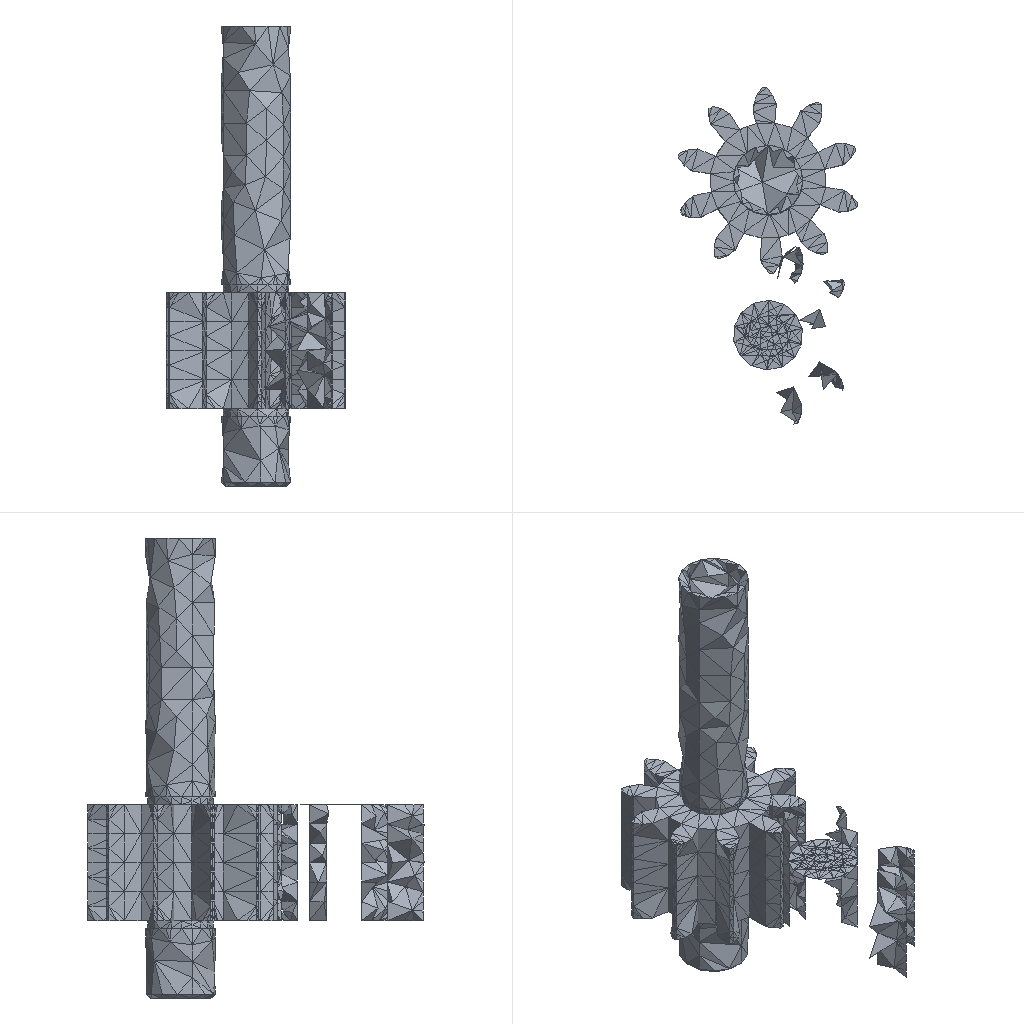Simulation study | ansys workbench
Ansys APDL input file, long lists of numbers shortened:
/batch
/config,noeldb,1     ! force off writing results to database
*get,_wallstrt,active,,time,wall
! ANSYS input file written by Workbench version 2022 R1
/assign,rstp,file,rst              ! Force Eigen analysis to write to file.rst because WB expects it
/solu
antype,,restart,,,perturbation
*DIM,_wb_ProjectScratch_dir_Modal,string,248
_wb_ProjectScratch_dir_Modal(1)= 'C:\_____\_____________\_______\_____\____\________________________\_______________\_______\_
*DIM,_wb_SolverFiles_dir_Modal,string,248
_wb_SolverFiles_dir_Modal(1)= 'C:\_____\_____________\_______\_____\____\________________________\___________\___\_____\____\_
*DIM,_wb_userfiles_dir_Modal,string,248
_wb_userfiles_dir_Modal(1)= 'C:\_____\_____________\_______\_____\____\________________________\___________\__________\_
/title,wbnew--__ (C5)
! ****** Begin Custom Load Command Snippet ******
/COM, ACT Extensions:
/COM,     LSDYNA, 2021.1
/COM,
! ****** End   Custom Load Command Snippet ******
perturb,modal,,CURRENT,DZEROKEEP          ! pre-stress modal analysis, only keep zero bcs in case future MSUP
solve, elform                                       ! Generate matrices needed for perturbation analysis
_thickRatio=0.75    ! Ratio of thick parts in the model
modopt,lanb,6
outres,erase
outres,all,none
outres,nsol,all
outres,etmp,all
mxpand                    ! default expand in case of complex solution
dmpopt,esav,no
dmpopt,emat,no
dmpopt,full,no
! *********** WB SOLVE COMMAND ***********
! check interactive state
*get,ANSINTER_,active,,int
*if,ANSINTER_,ne,0,then
/eof
*endif
solve
/com *************** Write FE CONNECTORS *********
CEWRITE,file,ce,,INTE
*get,_nmodalsolproc,active,0,numcpu
fini
/nopr
*get,_numnode,node,0,count
*get,_numelem,elem,0,count
*get, _MAXELEMNUM, elem, 0, NUM, MAX
*get, _MAXNODENUM, node, 0, NUM, MAX,,,INTERNAL
*get, _MAXELEMTYPE, etyp, 0, NUM, MAX
*get, _MAXREALCONST, real, 0, NUM, MAX
/gopr
*get,_wallasol,active,,time,wall
/post1
/nopr
*dim,_direction,CHAR,6,1
_direction(1) = 'X'
_direction(2) = 'Y'
_direction(3) = 'Z'
_direction(4) = 'ROTX'
_direction(5) = 'ROTY'
_direction(6) = 'ROTZ'
*get,_lastLS,active,0,set,LSTP
*get,_beginset,active,0,set,nset,first,_lastLS
*get,_endset,active,0,set,nset,last,_lastLS
_nummodes = 0
*if,_endset,gt,0,then
_nummodes = _endset - _beginset + 1
*endif
*do,i_mode,1,_nummodes
   *do,j_component,1,6
			*get,PFACT_%i_mode%_%j_component%,MODE,%i_mode%,PFACT,,DIREC,_direction(%j_component%)
   *enddo
*enddo
*dim,_tmdirection,CHAR,6,1
_tmdirection(1) = 'X'
_tmdirection(2) = 'Y'
_tmdirection(3) = 'Z'
_tmdirection(4) = 'X'
_tmdirection(5) = 'Y'
_tmdirection(6) = 'Z'
*do,j_component,1,6
    *if,j_component,gt,3,then
        *get,TOTALMASS_%j_component%,ELEM,0,IOR,_tmdirection(%j_component%)
    *else
        *get,TOTALMASS_%j_component%,ELEM,0,MTOT,_tmdirection(%j_component%)
    *endif
*enddo
/gopr
xmlo,ENCODING,ISO-8859-1
xmlo,parm
/xml,parm,xml
fini
/gopr
*get,_walldone,active,,time,wall
_preptime=(_wallbsol-_wallstrt)*3600
_solvtime=(_wallasol-_wallbsol)*3600
_posttime=(_walldone-_wallasol)*3600
_totaltim=(_walldone-_wallstrt)*3600
*get,_dlbratio,active,0,solu,dlbr
*get,_combtime,active,0,solu,comb
*get,_ssmode,active,0,solu,ssmm
*get,_ndofs,active,0,solu,ndof
/fclean				!clean distributed files
/com,--- Total number of nodes = %_numnode%
/com,--- Total number of elements = %_numelem%
/com,--- Element load balance ratio = %_dlbratio%
/com,--- Time to combine distributed files = %_combtime%
/com,--- Sparse memory mode = %_ssmode%
/com,--- Number of DOF = %_ndofs%
/wb,file,end               ! done with WB generated input